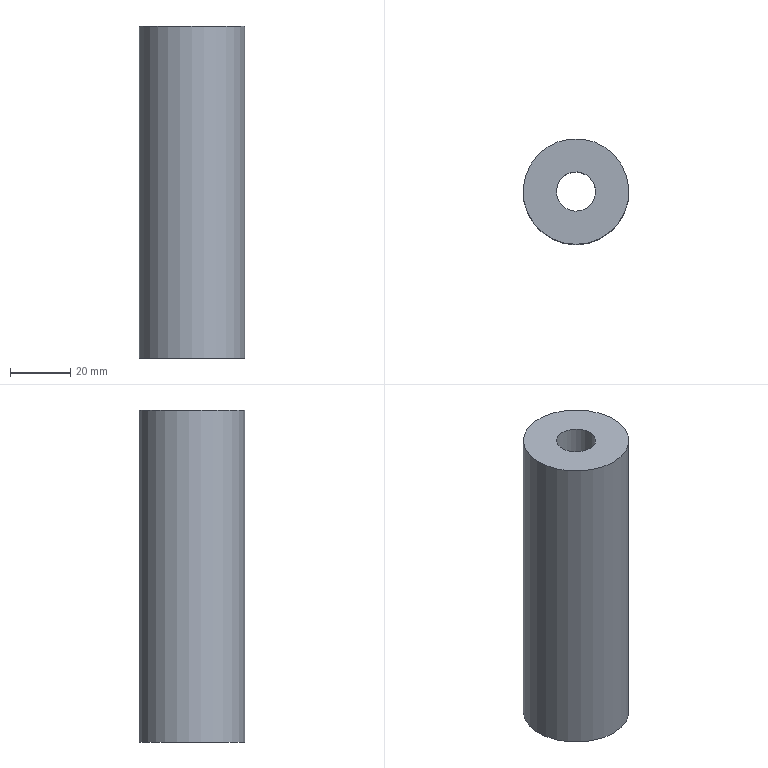Part | NX | features solid 2 | 1 solid | 6 faces | box 35 x 35 x 110 mm | volume 81253 mm3 | cylinder 3 | plane 3 | commonest cylinder face diameters 13 x1 20 x1 35 x1
STEP:
#1=CARTESIAN_POINT('',(-1020.617,366.961,-15.));
#2=VERTEX_POINT('',#1);
#3=CARTESIAN_POINT('',(-1037.852,370.,-15.));
#4=DIRECTION('',(0.,0.,1.));
#5=DIRECTION('',(0.9848,-0.1736,0.));
#6=AXIS2_PLACEMENT_3D('',#3,#4,#5);
#7=CIRCLE('',#6,17.5);
#8=EDGE_CURVE('',#2,#2,#7,.T.);
#9=ORIENTED_EDGE('',*,*,#8,.T.);
#10=EDGE_LOOP('',(#9));
#11=FACE_BOUND('',#10,.T.);
#12=CARTESIAN_POINT('',(-1020.617,366.961,95.));
#13=VERTEX_POINT('',#12);
#14=CARTESIAN_POINT('',(-1037.852,370.,95.));
#15=DIRECTION('',(0.,0.,1.));
#16=DIRECTION('',(0.9848,-0.1736,0.));
#17=AXIS2_PLACEMENT_3D('',#14,#15,#16);
#18=CIRCLE('',#17,17.5);
#19=EDGE_CURVE('',#13,#13,#18,.T.);
#20=ORIENTED_EDGE('',*,*,#19,.F.);
#21=EDGE_LOOP('',(#20));
#22=FACE_BOUND('',#21,.T.);
#23=CARTESIAN_POINT('',(-1037.852,370.,-15.));
#24=DIRECTION('',(0.,0.,1.));
#25=DIRECTION('',(0.9848,-0.1736,0.));
#26=AXIS2_PLACEMENT_3D('',#23,#24,#25);
#27=CYLINDRICAL_SURFACE('',#26,17.5);
#28=ADVANCED_FACE('',(#11,#22),#27,.T.);
#29=CARTESIAN_POINT('',(-1028.003,368.264,-15.));
#30=VERTEX_POINT('',#29);
#31=CARTESIAN_POINT('',(-1037.852,370.,-15.));
#32=DIRECTION('',(0.,0.,1.));
#33=DIRECTION('',(0.9848,-0.1736,0.));
#34=AXIS2_PLACEMENT_3D('',#31,#32,#33);
#35=CIRCLE('',#34,10.);
#36=EDGE_CURVE('',#30,#30,#35,.T.);
#37=ORIENTED_EDGE('',*,*,#36,.T.);
#38=EDGE_LOOP('',(#37));
#39=FACE_BOUND('',#38,.T.);
#40=ORIENTED_EDGE('',*,*,#8,.F.);
#41=EDGE_LOOP('',(#40));
#42=FACE_BOUND('',#41,.T.);
#43=CARTESIAN_POINT('',(-1037.852,370.,-15.));
#44=DIRECTION('',(0.,0.,1.));
#45=DIRECTION('',(0.9848,-0.1736,0.));
#46=AXIS2_PLACEMENT_3D('',#43,#44,#45);
#47=PLANE('',#46);
#48=ADVANCED_FACE('',(#39,#42),#47,.F.);
#49=CARTESIAN_POINT('',(-1031.45,368.871,95.));
#50=VERTEX_POINT('',#49);
#51=CARTESIAN_POINT('',(-1037.852,370.,95.));
#52=DIRECTION('',(0.,0.,1.));
#53=DIRECTION('',(0.9848,-0.1736,0.));
#54=AXIS2_PLACEMENT_3D('',#51,#52,#53);
#55=CIRCLE('',#54,6.5);
#56=EDGE_CURVE('',#50,#50,#55,.T.);
#57=ORIENTED_EDGE('',*,*,#56,.F.);
#58=EDGE_LOOP('',(#57));
#59=FACE_BOUND('',#58,.T.);
#60=ORIENTED_EDGE('',*,*,#19,.T.);
#61=EDGE_LOOP('',(#60));
#62=FACE_BOUND('',#61,.T.);
#63=CARTESIAN_POINT('',(-1037.852,370.,95.));
#64=DIRECTION('',(0.,0.,1.));
#65=DIRECTION('',(0.9848,-0.1736,0.));
#66=AXIS2_PLACEMENT_3D('',#63,#64,#65);
#67=PLANE('',#66);
#68=ADVANCED_FACE('',(#59,#62),#67,.T.);
#69=ORIENTED_EDGE('',*,*,#56,.T.);
#70=EDGE_LOOP('',(#69));
#71=FACE_BOUND('',#70,.T.);
#72=CARTESIAN_POINT('',(-1031.45,368.871,40.));
#73=VERTEX_POINT('',#72);
#74=CARTESIAN_POINT('',(-1037.852,370.,40.));
#75=DIRECTION('',(0.,0.,1.));
#76=DIRECTION('',(0.9848,-0.1736,0.));
#77=AXIS2_PLACEMENT_3D('',#74,#75,#76);
#78=CIRCLE('',#77,6.5);
#79=EDGE_CURVE('',#73,#73,#78,.T.);
#80=ORIENTED_EDGE('',*,*,#79,.F.);
#81=EDGE_LOOP('',(#80));
#82=FACE_BOUND('',#81,.T.);
#83=CARTESIAN_POINT('',(-1037.852,370.,485.));
#84=DIRECTION('',(0.,0.,1.));
#85=DIRECTION('',(0.9848,-0.1736,0.));
#86=AXIS2_PLACEMENT_3D('',#83,#84,#85);
#87=CYLINDRICAL_SURFACE('',#86,6.5);
#88=ADVANCED_FACE('',(#71,#82),#87,.F.);
#89=ORIENTED_EDGE('',*,*,#79,.T.);
#90=EDGE_LOOP('',(#89));
#91=FACE_BOUND('',#90,.T.);
#92=CARTESIAN_POINT('',(-1028.003,368.264,40.));
#93=VERTEX_POINT('',#92);
#94=CARTESIAN_POINT('',(-1037.852,370.,40.));
#95=DIRECTION('',(0.,0.,1.));
#96=DIRECTION('',(0.9848,-0.1736,0.));
#97=AXIS2_PLACEMENT_3D('',#94,#95,#96);
#98=CIRCLE('',#97,10.);
#99=EDGE_CURVE('',#93,#93,#98,.T.);
#100=ORIENTED_EDGE('',*,*,#99,.F.);
#101=EDGE_LOOP('',(#100));
#102=FACE_BOUND('',#101,.T.);
#103=CARTESIAN_POINT('',(-1037.852,370.,40.));
#104=DIRECTION('',(0.,0.,1.));
#105=DIRECTION('',(0.9848,-0.1736,0.));
#106=AXIS2_PLACEMENT_3D('',#103,#104,#105);
#107=PLANE('',#106);
#108=ADVANCED_FACE('',(#91,#102),#107,.F.);
#109=ORIENTED_EDGE('',*,*,#99,.T.);
#110=EDGE_LOOP('',(#109));
#111=FACE_BOUND('',#110,.T.);
#112=ORIENTED_EDGE('',*,*,#36,.F.);
#113=EDGE_LOOP('',(#112));
#114=FACE_BOUND('',#113,.T.);
#115=CARTESIAN_POINT('',(-1037.852,370.,-15.));
#116=DIRECTION('',(0.,0.,1.));
#117=DIRECTION('',(0.9848,-0.1736,0.));
#118=AXIS2_PLACEMENT_3D('',#115,#116,#117);
#119=CYLINDRICAL_SURFACE('',#118,10.);
#120=ADVANCED_FACE('',(#111,#114),#119,.F.);
#121=CLOSED_SHELL('',(#28,#48,#68,#88,#108,#120));
#122=MANIFOLD_SOLID_BREP('',#121);
#123=(LENGTH_UNIT()NAMED_UNIT(*)SI_UNIT(.MILLI.,.METRE.));
#124=UNCERTAINTY_MEASURE_WITH_UNIT(LENGTH_MEASURE(0.00001),#123,'','');
#125=(NAMED_UNIT(*)PLANE_ANGLE_UNIT()SI_UNIT($,.RADIAN.));
#126=(NAMED_UNIT(*)SI_UNIT($,.STERADIAN.)SOLID_ANGLE_UNIT());
#127=(GEOMETRIC_REPRESENTATION_CONTEXT(3)GLOBAL_UNCERTAINTY_ASSIGNED_CONTEXT((#124))GLOBAL_UNIT_ASSIGNED_CONTEXT((#123,#125,#126))REPRESENTATION_CONTEXT('',''));
#128=ADVANCED_BREP_SHAPE_REPRESENTATION('',(#122),#127);